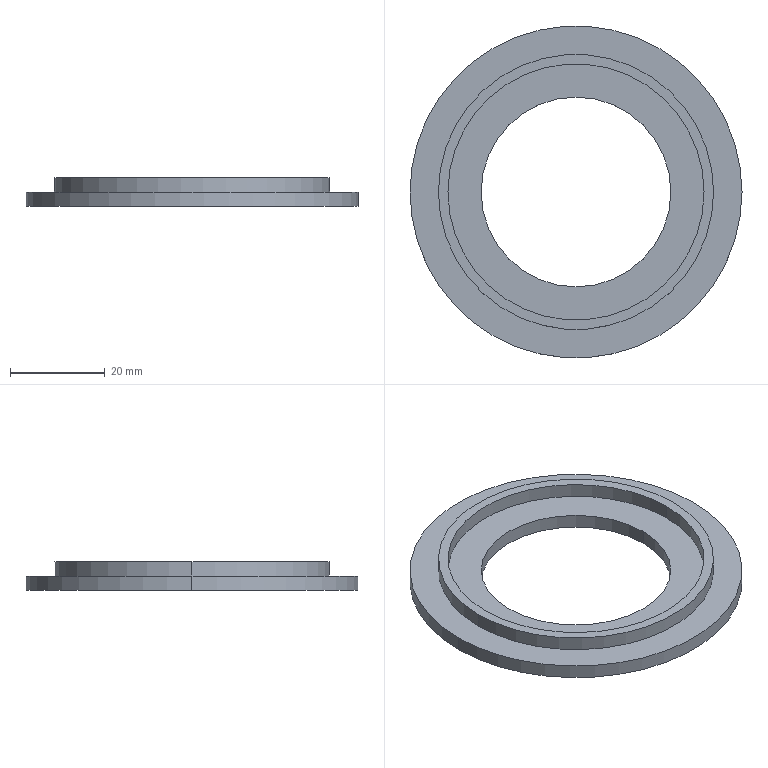Part | STEP file | outer seal2 | 1 solid | 12 faces | box 70 x 70 x 6 mm | volume 8831 mm3 | cylinder 8 | plane 4 | commonest cylinder face diameters 40 x2 54 x2 58 x2 70 x2
STEP:
#1=CARTESIAN_POINT('',(-20.,0.,0.));
#2=VERTEX_POINT('',#1);
#3=CARTESIAN_POINT('',(20.,0.,0.));
#4=VERTEX_POINT('',#3);
#5=CARTESIAN_POINT('',(0.,0.,0.));
#6=DIRECTION('',(0.,0.,1.));
#7=DIRECTION('',(1.,0.,0.));
#8=AXIS2_PLACEMENT_3D('',#5,#6,#7);
#9=CIRCLE('',#8,20.);
#10=EDGE_CURVE('',#2,#4,#9,.T.);
#11=ORIENTED_EDGE('',*,*,#10,.F.);
#12=CARTESIAN_POINT('',(-20.,0.,3.));
#13=VERTEX_POINT('',#12);
#14=CARTESIAN_POINT('',(-20.,0.,0.));
#15=DIRECTION('',(0.,0.,1.));
#16=VECTOR('',#15,1000.);
#17=LINE('',#14,#16);
#18=EDGE_CURVE('',#2,#13,#17,.T.);
#19=ORIENTED_EDGE('',*,*,#18,.T.);
#20=CARTESIAN_POINT('',(20.,0.,3.));
#21=VERTEX_POINT('',#20);
#22=CARTESIAN_POINT('',(0.,0.,3.));
#23=DIRECTION('',(0.,0.,1.));
#24=DIRECTION('',(1.,0.,0.));
#25=AXIS2_PLACEMENT_3D('',#22,#23,#24);
#26=CIRCLE('',#25,20.);
#27=EDGE_CURVE('',#13,#21,#26,.T.);
#28=ORIENTED_EDGE('',*,*,#27,.T.);
#29=CARTESIAN_POINT('',(20.,0.,0.));
#30=DIRECTION('',(0.,0.,1.));
#31=VECTOR('',#30,1000.);
#32=LINE('',#29,#31);
#33=EDGE_CURVE('',#4,#21,#32,.T.);
#34=ORIENTED_EDGE('',*,*,#33,.F.);
#35=EDGE_LOOP('',(#11,#19,#28,#34));
#36=FACE_OUTER_BOUND('',#35,.T.);
#37=CARTESIAN_POINT('',(0.,0.,0.));
#38=DIRECTION('',(0.,0.,1.));
#39=DIRECTION('',(1.,0.,0.));
#40=AXIS2_PLACEMENT_3D('',#37,#38,#39);
#41=CYLINDRICAL_SURFACE('',#40,20.);
#42=ADVANCED_FACE('',(#36),#41,.F.);
#43=CARTESIAN_POINT('',(-27.,0.,6.));
#44=VERTEX_POINT('',#43);
#45=CARTESIAN_POINT('',(27.,0.,6.));
#46=VERTEX_POINT('',#45);
#47=CARTESIAN_POINT('',(0.,0.,6.));
#48=DIRECTION('',(0.,0.,1.));
#49=DIRECTION('',(1.,0.,0.));
#50=AXIS2_PLACEMENT_3D('',#47,#48,#49);
#51=CIRCLE('',#50,27.);
#52=EDGE_CURVE('',#44,#46,#51,.T.);
#53=ORIENTED_EDGE('',*,*,#52,.T.);
#54=CARTESIAN_POINT('',(27.,0.,3.));
#55=VERTEX_POINT('',#54);
#56=CARTESIAN_POINT('',(27.,0.,6.));
#57=DIRECTION('',(0.,0.,-1.));
#58=VECTOR('',#57,1000.);
#59=LINE('',#56,#58);
#60=EDGE_CURVE('',#46,#55,#59,.T.);
#61=ORIENTED_EDGE('',*,*,#60,.T.);
#62=CARTESIAN_POINT('',(-27.,0.,3.));
#63=VERTEX_POINT('',#62);
#64=CARTESIAN_POINT('',(0.,0.,3.));
#65=DIRECTION('',(0.,0.,-1.));
#66=DIRECTION('',(1.,0.,0.));
#67=AXIS2_PLACEMENT_3D('',#64,#65,#66);
#68=CIRCLE('',#67,27.);
#69=EDGE_CURVE('',#55,#63,#68,.T.);
#70=ORIENTED_EDGE('',*,*,#69,.T.);
#71=CARTESIAN_POINT('',(-27.,0.,6.));
#72=DIRECTION('',(0.,0.,-1.));
#73=VECTOR('',#72,1000.);
#74=LINE('',#71,#73);
#75=EDGE_CURVE('',#44,#63,#74,.T.);
#76=ORIENTED_EDGE('',*,*,#75,.F.);
#77=EDGE_LOOP('',(#53,#61,#70,#76));
#78=FACE_OUTER_BOUND('',#77,.T.);
#79=CARTESIAN_POINT('',(0.,0.,6.));
#80=DIRECTION('',(0.,0.,-1.));
#81=DIRECTION('',(-1.,0.,0.));
#82=AXIS2_PLACEMENT_3D('',#79,#80,#81);
#83=CYLINDRICAL_SURFACE('',#82,27.);
#84=ADVANCED_FACE('',(#78),#83,.F.);
#85=CARTESIAN_POINT('',(29.,0.,6.));
#86=VERTEX_POINT('',#85);
#87=CARTESIAN_POINT('',(-29.,0.,6.));
#88=VERTEX_POINT('',#87);
#89=CARTESIAN_POINT('',(0.,0.,6.));
#90=DIRECTION('',(0.,0.,1.));
#91=DIRECTION('',(1.,0.,0.));
#92=AXIS2_PLACEMENT_3D('',#89,#90,#91);
#93=CIRCLE('',#92,29.);
#94=EDGE_CURVE('',#86,#88,#93,.T.);
#95=ORIENTED_EDGE('',*,*,#94,.F.);
#96=CARTESIAN_POINT('',(29.,0.,3.));
#97=VERTEX_POINT('',#96);
#98=CARTESIAN_POINT('',(29.,0.,6.));
#99=DIRECTION('',(0.,0.,-1.));
#100=VECTOR('',#99,1000.);
#101=LINE('',#98,#100);
#102=EDGE_CURVE('',#86,#97,#101,.T.);
#103=ORIENTED_EDGE('',*,*,#102,.T.);
#104=CARTESIAN_POINT('',(-29.,0.,3.));
#105=VERTEX_POINT('',#104);
#106=CARTESIAN_POINT('',(0.,0.,3.));
#107=DIRECTION('',(0.,0.,1.));
#108=DIRECTION('',(1.,0.,0.));
#109=AXIS2_PLACEMENT_3D('',#106,#107,#108);
#110=CIRCLE('',#109,29.);
#111=EDGE_CURVE('',#97,#105,#110,.T.);
#112=ORIENTED_EDGE('',*,*,#111,.T.);
#113=CARTESIAN_POINT('',(-29.,0.,6.));
#114=DIRECTION('',(0.,0.,-1.));
#115=VECTOR('',#114,1000.);
#116=LINE('',#113,#115);
#117=EDGE_CURVE('',#88,#105,#116,.T.);
#118=ORIENTED_EDGE('',*,*,#117,.F.);
#119=EDGE_LOOP('',(#95,#103,#112,#118));
#120=FACE_OUTER_BOUND('',#119,.T.);
#121=CARTESIAN_POINT('',(0.,0.,6.));
#122=DIRECTION('',(0.,0.,-1.));
#123=DIRECTION('',(-1.,0.,0.));
#124=AXIS2_PLACEMENT_3D('',#121,#122,#123);
#125=CYLINDRICAL_SURFACE('',#124,29.);
#126=ADVANCED_FACE('',(#120),#125,.T.);
#127=CARTESIAN_POINT('',(35.,0.,3.));
#128=VERTEX_POINT('',#127);
#129=CARTESIAN_POINT('',(-35.,0.,3.));
#130=VERTEX_POINT('',#129);
#131=CARTESIAN_POINT('',(0.,0.,3.));
#132=DIRECTION('',(0.,0.,1.));
#133=DIRECTION('',(1.,0.,0.));
#134=AXIS2_PLACEMENT_3D('',#131,#132,#133);
#135=CIRCLE('',#134,35.);
#136=EDGE_CURVE('',#128,#130,#135,.T.);
#137=ORIENTED_EDGE('',*,*,#136,.F.);
#138=CARTESIAN_POINT('',(35.,0.,0.));
#139=VERTEX_POINT('',#138);
#140=CARTESIAN_POINT('',(35.,0.,3.));
#141=DIRECTION('',(0.,0.,-1.));
#142=VECTOR('',#141,1000.);
#143=LINE('',#140,#142);
#144=EDGE_CURVE('',#128,#139,#143,.T.);
#145=ORIENTED_EDGE('',*,*,#144,.T.);
#146=CARTESIAN_POINT('',(-35.,0.,0.));
#147=VERTEX_POINT('',#146);
#148=CARTESIAN_POINT('',(0.,0.,0.));
#149=DIRECTION('',(0.,0.,1.));
#150=DIRECTION('',(1.,0.,0.));
#151=AXIS2_PLACEMENT_3D('',#148,#149,#150);
#152=CIRCLE('',#151,35.);
#153=EDGE_CURVE('',#139,#147,#152,.T.);
#154=ORIENTED_EDGE('',*,*,#153,.T.);
#155=CARTESIAN_POINT('',(-35.,0.,3.));
#156=DIRECTION('',(0.,0.,-1.));
#157=VECTOR('',#156,1000.);
#158=LINE('',#155,#157);
#159=EDGE_CURVE('',#130,#147,#158,.T.);
#160=ORIENTED_EDGE('',*,*,#159,.F.);
#161=EDGE_LOOP('',(#137,#145,#154,#160));
#162=FACE_OUTER_BOUND('',#161,.T.);
#163=CARTESIAN_POINT('',(0.,0.,3.));
#164=DIRECTION('',(0.,0.,-1.));
#165=DIRECTION('',(-1.,0.,0.));
#166=AXIS2_PLACEMENT_3D('',#163,#164,#165);
#167=CYLINDRICAL_SURFACE('',#166,35.);
#168=ADVANCED_FACE('',(#162),#167,.T.);
#169=ORIENTED_EDGE('',*,*,#144,.F.);
#170=CARTESIAN_POINT('',(0.,0.,3.));
#171=DIRECTION('',(0.,0.,1.));
#172=DIRECTION('',(1.,0.,0.));
#173=AXIS2_PLACEMENT_3D('',#170,#171,#172);
#174=CIRCLE('',#173,35.);
#175=EDGE_CURVE('',#130,#128,#174,.T.);
#176=ORIENTED_EDGE('',*,*,#175,.F.);
#177=ORIENTED_EDGE('',*,*,#159,.T.);
#178=CARTESIAN_POINT('',(0.,0.,0.));
#179=DIRECTION('',(0.,0.,1.));
#180=DIRECTION('',(1.,0.,0.));
#181=AXIS2_PLACEMENT_3D('',#178,#179,#180);
#182=CIRCLE('',#181,35.);
#183=EDGE_CURVE('',#147,#139,#182,.T.);
#184=ORIENTED_EDGE('',*,*,#183,.T.);
#185=EDGE_LOOP('',(#169,#176,#177,#184));
#186=FACE_OUTER_BOUND('',#185,.T.);
#187=CARTESIAN_POINT('',(0.,0.,3.));
#188=DIRECTION('',(0.,0.,-1.));
#189=DIRECTION('',(-1.,0.,0.));
#190=AXIS2_PLACEMENT_3D('',#187,#188,#189);
#191=CYLINDRICAL_SURFACE('',#190,35.);
#192=ADVANCED_FACE('',(#186),#191,.T.);
#193=CARTESIAN_POINT('',(0.,0.,3.));
#194=DIRECTION('',(0.,0.,1.));
#195=DIRECTION('',(1.,0.,0.));
#196=AXIS2_PLACEMENT_3D('',#193,#194,#195);
#197=CIRCLE('',#196,29.);
#198=EDGE_CURVE('',#105,#97,#197,.T.);
#199=ORIENTED_EDGE('',*,*,#198,.F.);
#200=ORIENTED_EDGE('',*,*,#111,.F.);
#201=EDGE_LOOP('',(#199,#200));
#202=FACE_BOUND('',#201,.T.);
#203=ORIENTED_EDGE('',*,*,#175,.T.);
#204=ORIENTED_EDGE('',*,*,#136,.T.);
#205=EDGE_LOOP('',(#203,#204));
#206=FACE_OUTER_BOUND('',#205,.T.);
#207=CARTESIAN_POINT('',(0.,0.,3.));
#208=DIRECTION('',(0.,0.,1.));
#209=DIRECTION('',(1.,0.,0.));
#210=AXIS2_PLACEMENT_3D('',#207,#208,#209);
#211=PLANE('',#210);
#212=ADVANCED_FACE('',(#202,#206),#211,.T.);
#213=CARTESIAN_POINT('',(0.,0.,0.));
#214=DIRECTION('',(0.,0.,1.));
#215=DIRECTION('',(1.,0.,0.));
#216=AXIS2_PLACEMENT_3D('',#213,#214,#215);
#217=CIRCLE('',#216,20.);
#218=EDGE_CURVE('',#4,#2,#217,.T.);
#219=ORIENTED_EDGE('',*,*,#218,.T.);
#220=ORIENTED_EDGE('',*,*,#10,.T.);
#221=EDGE_LOOP('',(#219,#220));
#222=FACE_BOUND('',#221,.T.);
#223=ORIENTED_EDGE('',*,*,#183,.F.);
#224=ORIENTED_EDGE('',*,*,#153,.F.);
#225=EDGE_LOOP('',(#223,#224));
#226=FACE_OUTER_BOUND('',#225,.T.);
#227=CARTESIAN_POINT('',(0.,0.,0.));
#228=DIRECTION('',(0.,0.,1.));
#229=DIRECTION('',(1.,0.,0.));
#230=AXIS2_PLACEMENT_3D('',#227,#228,#229);
#231=PLANE('',#230);
#232=ADVANCED_FACE('',(#222,#226),#231,.F.);
#233=CARTESIAN_POINT('',(0.,0.,6.));
#234=DIRECTION('',(0.,0.,1.));
#235=DIRECTION('',(1.,0.,0.));
#236=AXIS2_PLACEMENT_3D('',#233,#234,#235);
#237=CIRCLE('',#236,29.);
#238=EDGE_CURVE('',#88,#86,#237,.T.);
#239=ORIENTED_EDGE('',*,*,#238,.T.);
#240=ORIENTED_EDGE('',*,*,#94,.T.);
#241=EDGE_LOOP('',(#239,#240));
#242=FACE_OUTER_BOUND('',#241,.T.);
#243=ORIENTED_EDGE('',*,*,#52,.F.);
#244=CARTESIAN_POINT('',(0.,0.,6.));
#245=DIRECTION('',(0.,0.,1.));
#246=DIRECTION('',(1.,0.,0.));
#247=AXIS2_PLACEMENT_3D('',#244,#245,#246);
#248=CIRCLE('',#247,27.);
#249=EDGE_CURVE('',#46,#44,#248,.T.);
#250=ORIENTED_EDGE('',*,*,#249,.F.);
#251=EDGE_LOOP('',(#243,#250));
#252=FACE_BOUND('',#251,.T.);
#253=CARTESIAN_POINT('',(0.,0.,6.));
#254=DIRECTION('',(0.,0.,1.));
#255=DIRECTION('',(1.,0.,0.));
#256=AXIS2_PLACEMENT_3D('',#253,#254,#255);
#257=PLANE('',#256);
#258=ADVANCED_FACE('',(#242,#252),#257,.T.);
#259=ORIENTED_EDGE('',*,*,#102,.F.);
#260=ORIENTED_EDGE('',*,*,#238,.F.);
#261=ORIENTED_EDGE('',*,*,#117,.T.);
#262=ORIENTED_EDGE('',*,*,#198,.T.);
#263=EDGE_LOOP('',(#259,#260,#261,#262));
#264=FACE_OUTER_BOUND('',#263,.T.);
#265=CARTESIAN_POINT('',(0.,0.,6.));
#266=DIRECTION('',(0.,0.,-1.));
#267=DIRECTION('',(-1.,0.,0.));
#268=AXIS2_PLACEMENT_3D('',#265,#266,#267);
#269=CYLINDRICAL_SURFACE('',#268,29.);
#270=ADVANCED_FACE('',(#264),#269,.T.);
#271=ORIENTED_EDGE('',*,*,#60,.F.);
#272=ORIENTED_EDGE('',*,*,#249,.T.);
#273=ORIENTED_EDGE('',*,*,#75,.T.);
#274=CARTESIAN_POINT('',(0.,0.,3.));
#275=DIRECTION('',(0.,0.,-1.));
#276=DIRECTION('',(1.,0.,0.));
#277=AXIS2_PLACEMENT_3D('',#274,#275,#276);
#278=CIRCLE('',#277,27.);
#279=EDGE_CURVE('',#63,#55,#278,.T.);
#280=ORIENTED_EDGE('',*,*,#279,.T.);
#281=EDGE_LOOP('',(#271,#272,#273,#280));
#282=FACE_OUTER_BOUND('',#281,.T.);
#283=CARTESIAN_POINT('',(0.,0.,6.));
#284=DIRECTION('',(0.,0.,-1.));
#285=DIRECTION('',(-1.,0.,0.));
#286=AXIS2_PLACEMENT_3D('',#283,#284,#285);
#287=CYLINDRICAL_SURFACE('',#286,27.);
#288=ADVANCED_FACE('',(#282),#287,.F.);
#289=CARTESIAN_POINT('',(0.,0.,3.));
#290=DIRECTION('',(0.,0.,1.));
#291=DIRECTION('',(1.,0.,0.));
#292=AXIS2_PLACEMENT_3D('',#289,#290,#291);
#293=CIRCLE('',#292,20.);
#294=EDGE_CURVE('',#21,#13,#293,.T.);
#295=ORIENTED_EDGE('',*,*,#294,.F.);
#296=ORIENTED_EDGE('',*,*,#27,.F.);
#297=EDGE_LOOP('',(#295,#296));
#298=FACE_BOUND('',#297,.T.);
#299=ORIENTED_EDGE('',*,*,#279,.F.);
#300=ORIENTED_EDGE('',*,*,#69,.F.);
#301=EDGE_LOOP('',(#299,#300));
#302=FACE_OUTER_BOUND('',#301,.T.);
#303=CARTESIAN_POINT('',(0.,0.,3.));
#304=DIRECTION('',(0.,0.,1.));
#305=DIRECTION('',(1.,0.,0.));
#306=AXIS2_PLACEMENT_3D('',#303,#304,#305);
#307=PLANE('',#306);
#308=ADVANCED_FACE('',(#298,#302),#307,.T.);
#309=ORIENTED_EDGE('',*,*,#18,.F.);
#310=ORIENTED_EDGE('',*,*,#218,.F.);
#311=ORIENTED_EDGE('',*,*,#33,.T.);
#312=ORIENTED_EDGE('',*,*,#294,.T.);
#313=EDGE_LOOP('',(#309,#310,#311,#312));
#314=FACE_OUTER_BOUND('',#313,.T.);
#315=CARTESIAN_POINT('',(0.,0.,0.));
#316=DIRECTION('',(0.,0.,1.));
#317=DIRECTION('',(1.,0.,0.));
#318=AXIS2_PLACEMENT_3D('',#315,#316,#317);
#319=CYLINDRICAL_SURFACE('',#318,20.);
#320=ADVANCED_FACE('',(#314),#319,.F.);
#321=CLOSED_SHELL('',(#42,#84,#126,#168,#192,#212,#232,#258,#270,#288,#308,#320));
#322=MANIFOLD_SOLID_BREP('',#321);
#323=CARTESIAN_POINT('',(0.,0.,0.));
#324=DIRECTION('',(0.,0.,1.));
#325=DIRECTION('',(1.,0.,0.));
#326=AXIS2_PLACEMENT_3D('',#323,#324,#325);
#327=(LENGTH_UNIT()NAMED_UNIT(*)SI_UNIT(.MILLI.,.METRE.));
#328=UNCERTAINTY_MEASURE_WITH_UNIT(LENGTH_MEASURE(0.00001),#327,'','');
#329=(NAMED_UNIT(*)PLANE_ANGLE_UNIT()SI_UNIT($,.RADIAN.));
#330=(NAMED_UNIT(*)SI_UNIT($,.STERADIAN.)SOLID_ANGLE_UNIT());
#331=(GEOMETRIC_REPRESENTATION_CONTEXT(3)GLOBAL_UNCERTAINTY_ASSIGNED_CONTEXT((#328))GLOBAL_UNIT_ASSIGNED_CONTEXT((#327,#329,#330))REPRESENTATION_CONTEXT('',''));
#332=ADVANCED_BREP_SHAPE_REPRESENTATION('',(#322,#326),#331);